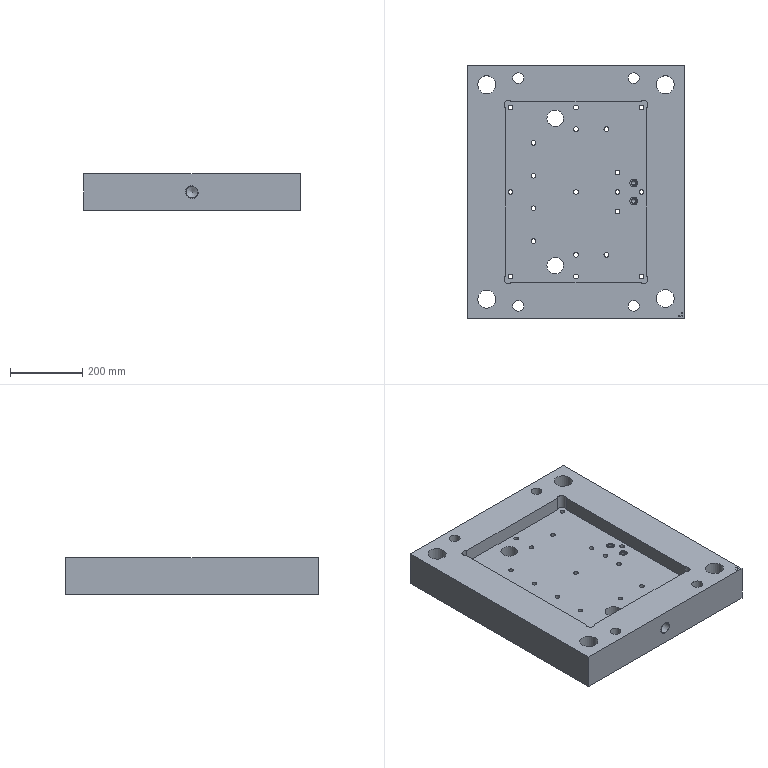Part | NX | features 模具.stp<1>[6] 2 | 1 solid | 174 faces | box 600 x 700 x 100 mm | volume 32062789 mm3 | cylinder 88 | plane 74 | cone 12 | commonest cylinder face diameters 13 x20 20 x14 30 x8 17.5 x6 19.7 x6 24 x6